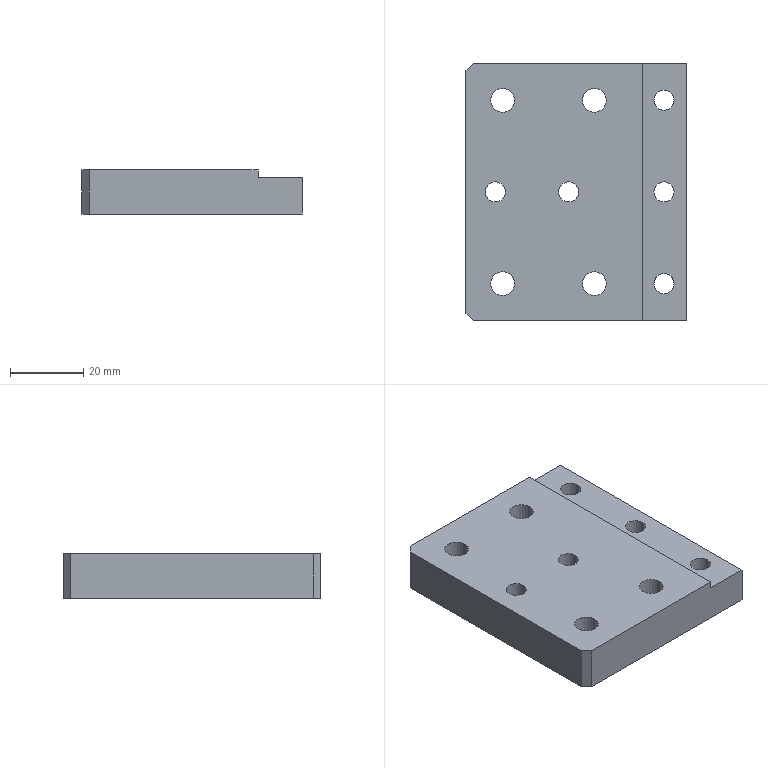Part | STEP file | PN_0059 Mount electronic clip mounting base plate A | 1 solid | 43 faces | box 60 x 70 x 12 mm | volume 44235 mm3 | cylinder 28 | plane 15 | commonest cylinder face diameters 5.5 x10 10 x10 6.5 x8